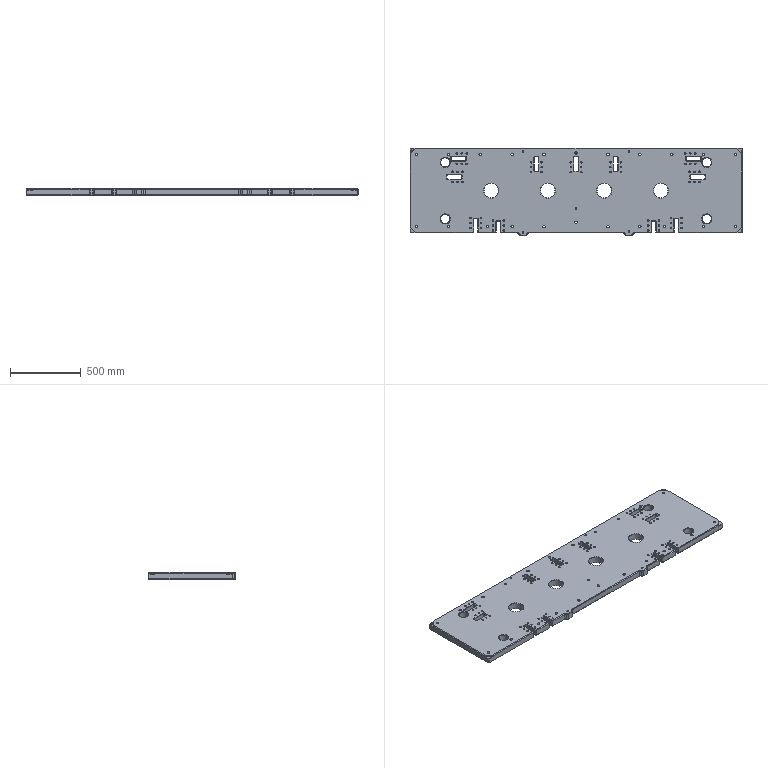Part | STEP file | solid 227 | 1 solid | 744 faces | box 2350 x 620 x 50 mm | volume 65620843 mm3 | plane 315 | cylinder 259 | cone 170 | commonest cylinder face diameters 14 x45 11 x44 18 x44 5 x30 26 x30 10 x22